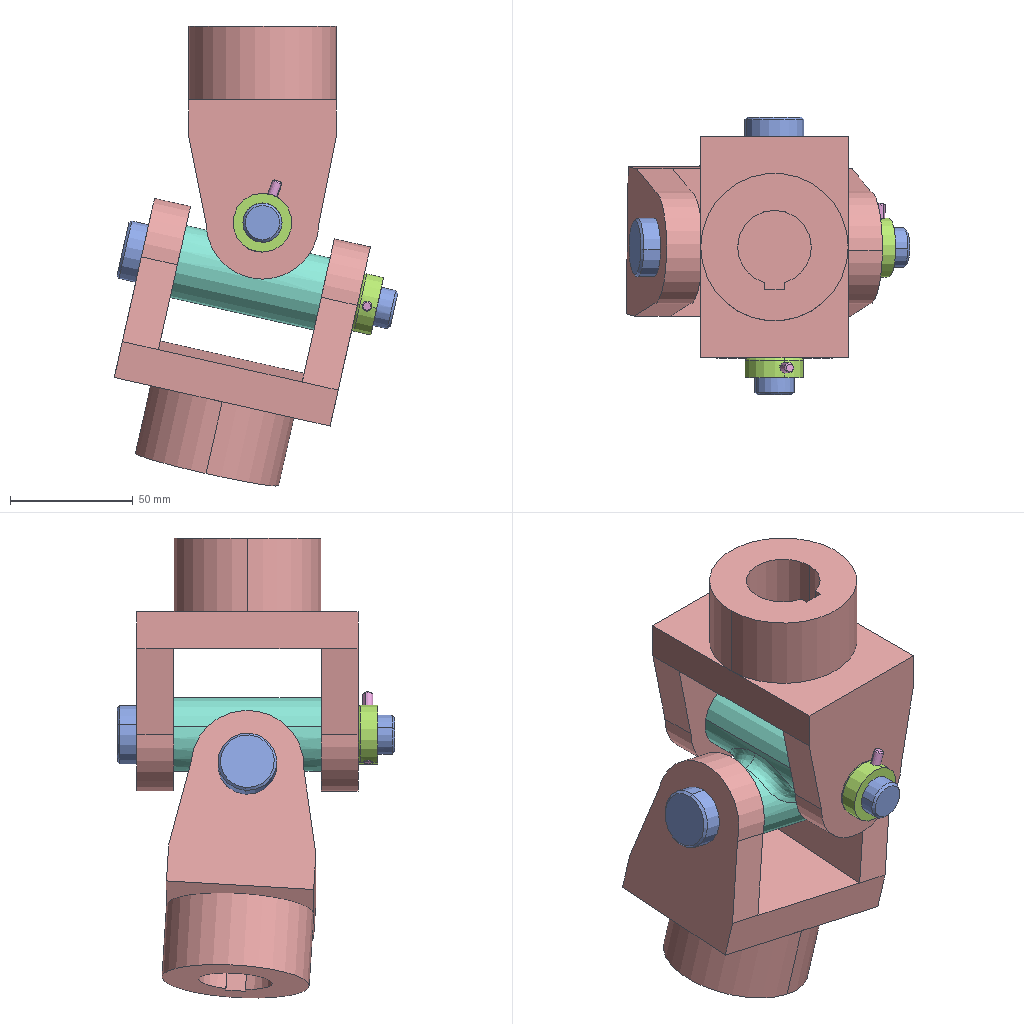Assembly | SolidWorks | 5 different items | 9 placed | box 115 x 113 x 187 mm
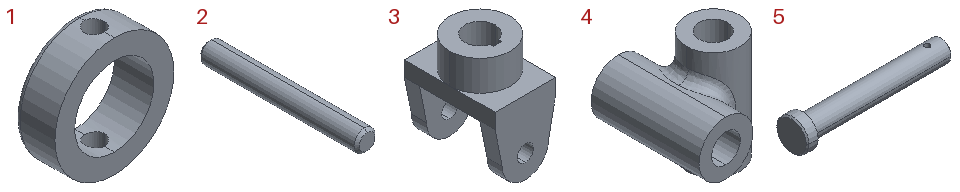Parts list (item | quantity | size | volume | features):
1 | x2 | 24 x 8 x 24 mm | 1894 mm3 | features Extrusion 1, Fillet 1, ICE 1
2 | x2 | 4 x 30 x 4 mm | 374.111 mm3 | features Chamfer 1, Extrusion 1
3 | x2 | 60 x 90 x 103 mm | 218531 mm3 | features ICE 2, Extrusion 1, MirrorPattern 1
4 | x1 | 53 x 60 x 60 mm | 59937 mm3 | features Extrusion 1, Fillet 1, ICE 1
5 | x2 | 113 x 24 x 24 mm | 24470 mm3 | features Chamfer 2, ICE 1, Revolution 1
Mates (type | each side: item.copy, entity, surface, feature):
Concentric | 3.1 face cylinder Boss-Extrude2 | 4.1 face cylinder Boss-Extrude1
Coincident | 3.1 face plane Mirror1 | 4.1 edge
Coincident | 4.1 face cylinder Boss-Extrude2 | 3.2 edge
Coincident | 4.1 face plane Boss-Extrude2 | 3.2 edge
Coincident | 3.1 edge | 5.1 face cylinder Revolve1
Coincident | 3.1 face plane Boss-Extrude1 | 5.1 edge
Coincident | 3.2 edge | 5.2 face cylinder Revolve1
Coincident | 3.2 face plane Boss-Extrude1 | 5.2 edge
Concentric | 5.2 face cylinder Revolve1 | 1.1 face cylinder Boss-Extrude1
Coincident | 3.2 face plane Boss-Extrude1 | 1.1 edge
Concentric | 5.2 face cylinder Cut-Extrude1 | 1.1 face cylinder Cut-Extrude1
Concentric | 5.2 face cylinder Cut-Extrude1 | 2.1 face cylinder Boss-Extrude1
Tangent | 1.1 face cylinder Boss-Extrude1 | 2.1 face plane Boss-Extrude1
Concentric | 5.1 face cylinder Revolve1 | 1.2 face cylinder Boss-Extrude1
Coincident | 3.1 face plane Boss-Extrude1 | 1.2 edge
Concentric | 5.1 face cylinder Cut-Extrude1 | 1.2 face cylinder Cut-Extrude1
Concentric | 5.1 face cylinder Cut-Extrude1 | 2.2 face cylinder Boss-Extrude1
Tangent | 1.2 face cylinder Boss-Extrude1 | 2.2 face plane Boss-Extrude1